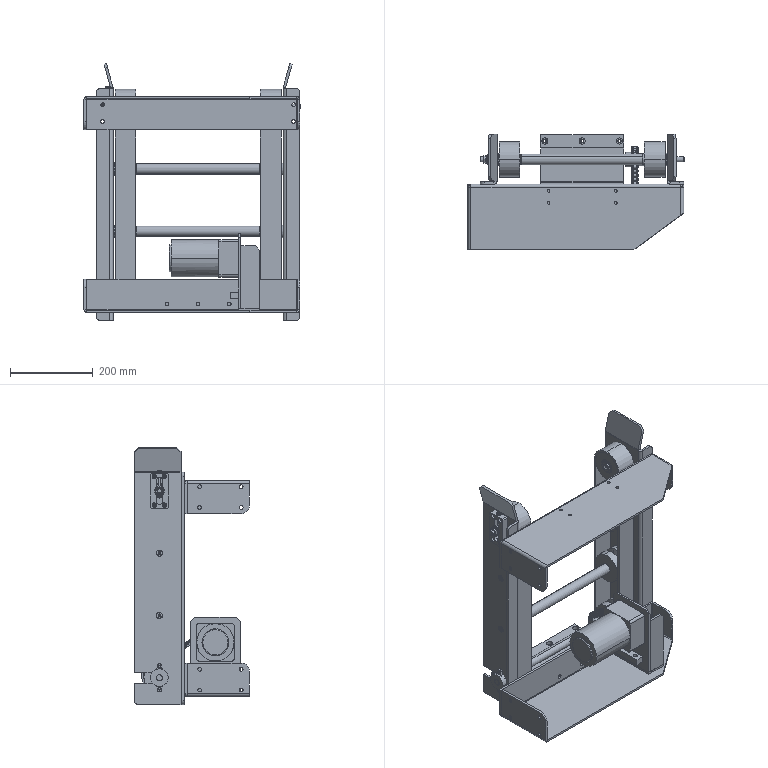Part | SolidWorks | features CompositeCurve 14, InContextFeatHolder 6, ReferencePattern 5, LocalLPattern 1 | 104 solids | 3019 faces | volume 6635469 mm3 | cylinder 1542 | plane 759 | cone 264 | sphere 256 | torus 192 | spline 6 | commonest cylinder face diameters 4.45 x288 11.81 x216 57.066 x144 8.51 x72 9 x72 15 x62